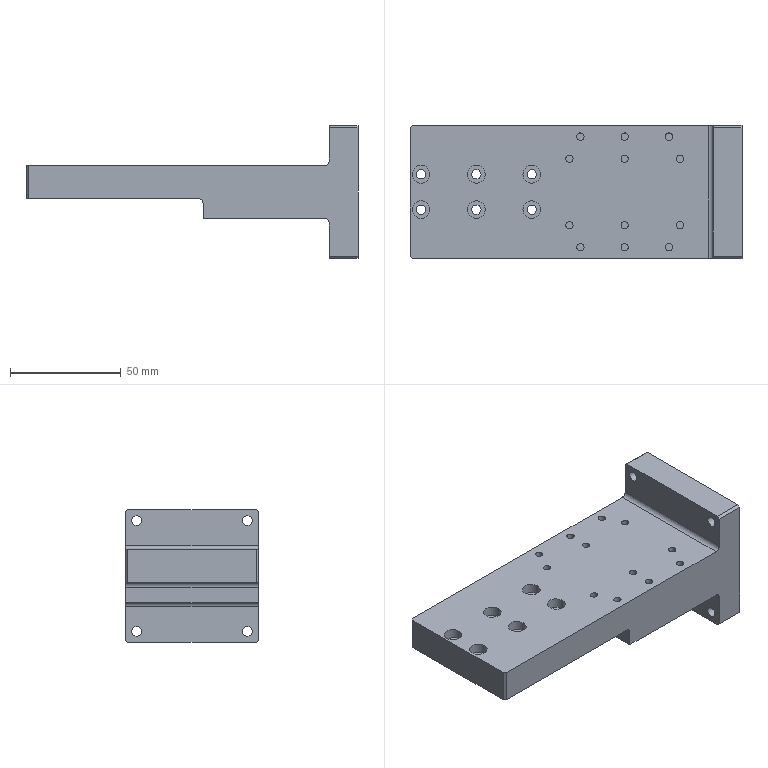NC program | NX | posted with a generic post | part box 150 x 60 x 60 mm
Whole program:
N10 G17 G21 G94 G90
(FLOOR_WALL_COPY , TOOL : D80)
N12 T19 M6
N14 G54
N16 G17 G0 G90 X120. Y0. B0. C0. S6500 M3
N18 G43 Z30. H19
N20 Z7.
N22 G94 G1 Z4. F1500.
N24 X117.
N26 X-117.
N28 X-120.
N30 Z7.
N32 G0 Z30.
N34 X120.
N36 Z6.
N38 G1 Z3.
N40 X117.
N42 X-117.
N44 X-120.
N46 Z6.
N48 G0 Z30.
N50 X120.
N52 Z5.
N54 G1 Z2.
N56 X117.
N58 X-117.
N60 X-120.
N62 Z5.
N64 G0 Z30.
N66 X120.
N68 Z4.
N70 G1 Z1.
N72 X117.
N74 X-117.
N76 X-120.
N78 Z4.
N80 G0 Z30.
N82 X120.
N84 Z3.
N86 G1 Z0.
N88 X117.
N90 X-117.
N92 X-120.
N94 Z3.
N96 G0 Z30.
N98 M5
(PLANAR_MILL_COPY , TOOL : D10)
N100 T15 M6
N102 G54
N104 G17 G0 G90 X-3.6 Y-31.732 B0. C0. S9500 M3
N106 G43 Z30. H15
N108 Z-23.8
N110 G94 G1 Z-24.8 F1000.
N112 X-2.1 Y-30.866
N114 G3 X-1.6 Y-30. R1.
N116 G1 Y30. F2500.
N118 G3 X-2.1 Y30.866 R1.
N120 G1 X-3.6 Y31.732
N122 Z-23.8
N124 G0 Z30.
N126 Y-32.021
N128 Z-23.8
N130 G1 Z-24.8 F1000.
N132 X-1.6 Y-30.866
N134 G3 X-1.1 Y-30. R1.
N136 G1 Y30. F2500.
N138 G3 X-1.6 Y30.866 R1.
N140 G1 X-3.6 Y32.021
N142 Z-23.8
N144 G0 Z30.
N146 Y-32.309
N148 Z-23.8
N150 G1 Z-24.8 F1000.
N152 X-1.1 Y-30.866
N154 G3 X-0.6 Y-30. R1.
N156 G1 Y30. F2500.
N158 G3 X-1.1 Y30.866 R1.
N160 G1 X-3.6 Y32.309
N162 Z-23.8
N164 G0 Z30.
N166 Y-32.598
N168 Z-23.8
N170 G1 Z-24.8 F1000.
N172 X-0.6 Y-30.866
N174 G3 X-0.1 Y-30. R1.
N176 G1 Y30. F2500.
N178 G3 X-0.6 Y30.866 R1.
N180 G1 X-3.6 Y32.598
N182 Z-23.8
N184 G0 Z30.
(PLANAR_MILL_COPY_COPY , TOOL : D10)
N186 X53.4 Y-30.732
N188 Z-14.8
N190 G1 Z-15.8 F1000.
N192 X54.9 Y-29.866
N194 G3 X55.4 Y-29. R1.
N196 G1 Y29. F2500.
N198 G3 X54.9 Y29.866 R1.
N200 G1 X53.4 Y30.732
N202 Z-14.8
N204 G0 Z30.
N206 Y-31.021
N208 Z-14.8
N210 G1 Z-15.8 F1000.
N212 X55.4 Y-29.866
N214 G3 X55.9 Y-29. R1.
N216 G1 Y29. F2500.
N218 G3 X55.4 Y29.866 R1.
N220 G1 X53.4 Y31.021
N222 Z-14.8
N224 G0 Z30.
N226 Y-31.309
N228 Z-14.8
N230 G1 Z-15.8 F1000.
N232 X55.9 Y-29.866
N234 G3 X56.4 Y-29. R1.
N236 G1 Y29. F2500.
N238 G3 X55.9 Y29.866 R1.
N240 G1 X53.4 Y31.309
N242 Z-14.8
N244 G0 Z30.
N246 Y-31.598
N248 Z-14.8
N250 G1 Z-15.8 F1000.
N252 X56.4 Y-29.866
N254 G3 X56.9 Y-29. R1.
N256 G1 Y29. F2500.
N258 G3 X56.4 Y29.866 R1.
N260 G1 X53.4 Y31.598
N262 Z-14.8
N264 G0 Z30.
N266 M5
(FLOOR_WALL_1_COPY_COPY , TOOL : D10JING)
N268 T14 M6
N270 G54
N272 G17 G0 G90 X5.001 Y-38. B0. C0. S9500 M3
N274 G43 Z30. H14
N276 Z-15.
N278 G94 G1 Z-18. F1000.
N280 Y-35.
N282 Y35. F1500.
N284 X9.951
N286 Y-35.
N288 X14.901
N290 Y35.
N292 X19.851
N294 Y-35.
N296 X24.801
N298 Y35.
N300 X29.75
N302 Y-35.
N304 X34.7
N306 Y35.
N308 X39.65
N310 Y-35.
N312 X44.6
N314 Y35.
N316 X49.55
N318 Y-35.
N320 X54.5
N322 Y35.
N324 Y38.
N326 Z-15.
N328 G0 Z30.
N330 X55. Y-38.
N332 Z-15.
N334 G1 Z-18. F1000.
N336 Y-35.
N338 Y35. F1500.
N340 Y38.
N342 Z-15.
N344 G0 Z30.
N346 X-74.999 Y-38.
N348 Z-24.
N350 G1 Z-27. F1000.
N352 Y-35.
N354 Y35. F1500.
N356 X-70.166
N358 Y-35.
N360 X-65.332
N362 Y35.
N364 X-60.499
N366 Y-35.
N368 X-55.666
N370 Y35.
N372 X-50.833
N374 Y-35.
N376 X-45.999
N378 Y35.
N380 X-41.166
N382 Y-35.
N384 X-36.333
N386 Y35.
N388 X-31.5
N390 Y-35.
N392 X-26.666
N394 Y35.
N396 X-21.833
N398 Y-35.
N400 X-17.
N402 Y35.
N404 X-12.167
N406 Y-35.
N408 X-7.333
N410 Y35.
N412 X-2.5
N414 Y-35.
N416 Y-38.
N418 Z-24.
N420 G0 Z30.
N422 X-2.
N424 Z-24.
N426 G1 Z-27. F1000.
N428 Y-35.
N430 Y35. F1500.
N432 Y38.
N434 Z-24.
N436 G0 Z30.
N438 M5
N440 M2